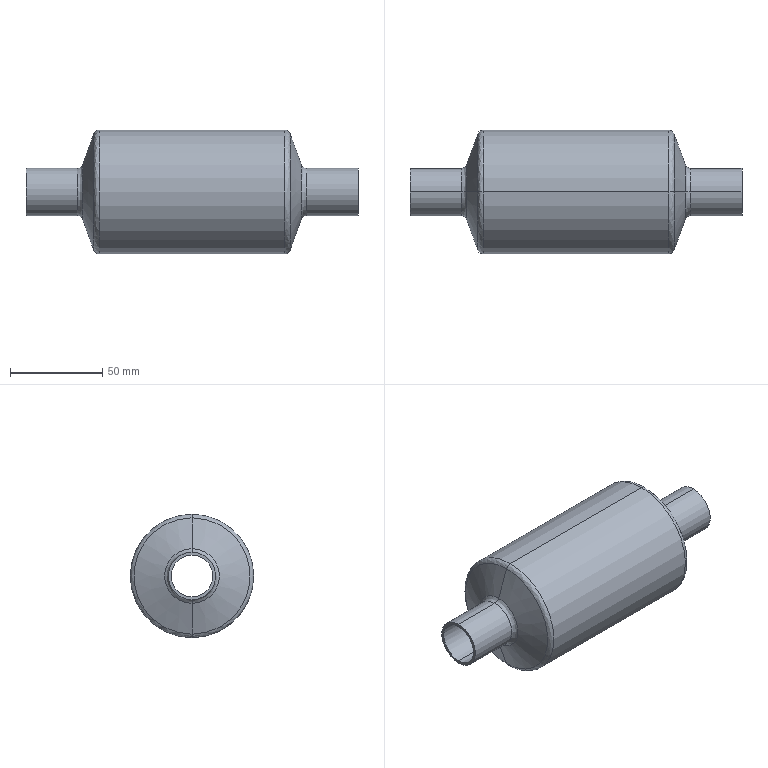Part | STEP file | EK-167S-seven-eighths filter | 1 solid | 30 faces | box 180 x 67 x 67 mm | volume 48133 mm3 | cylinder 12 | spline 8 | cone 8 | plane 2 | commonest cylinder face diameters 22.7 x4 25.7 x4 64 x2 67 x2